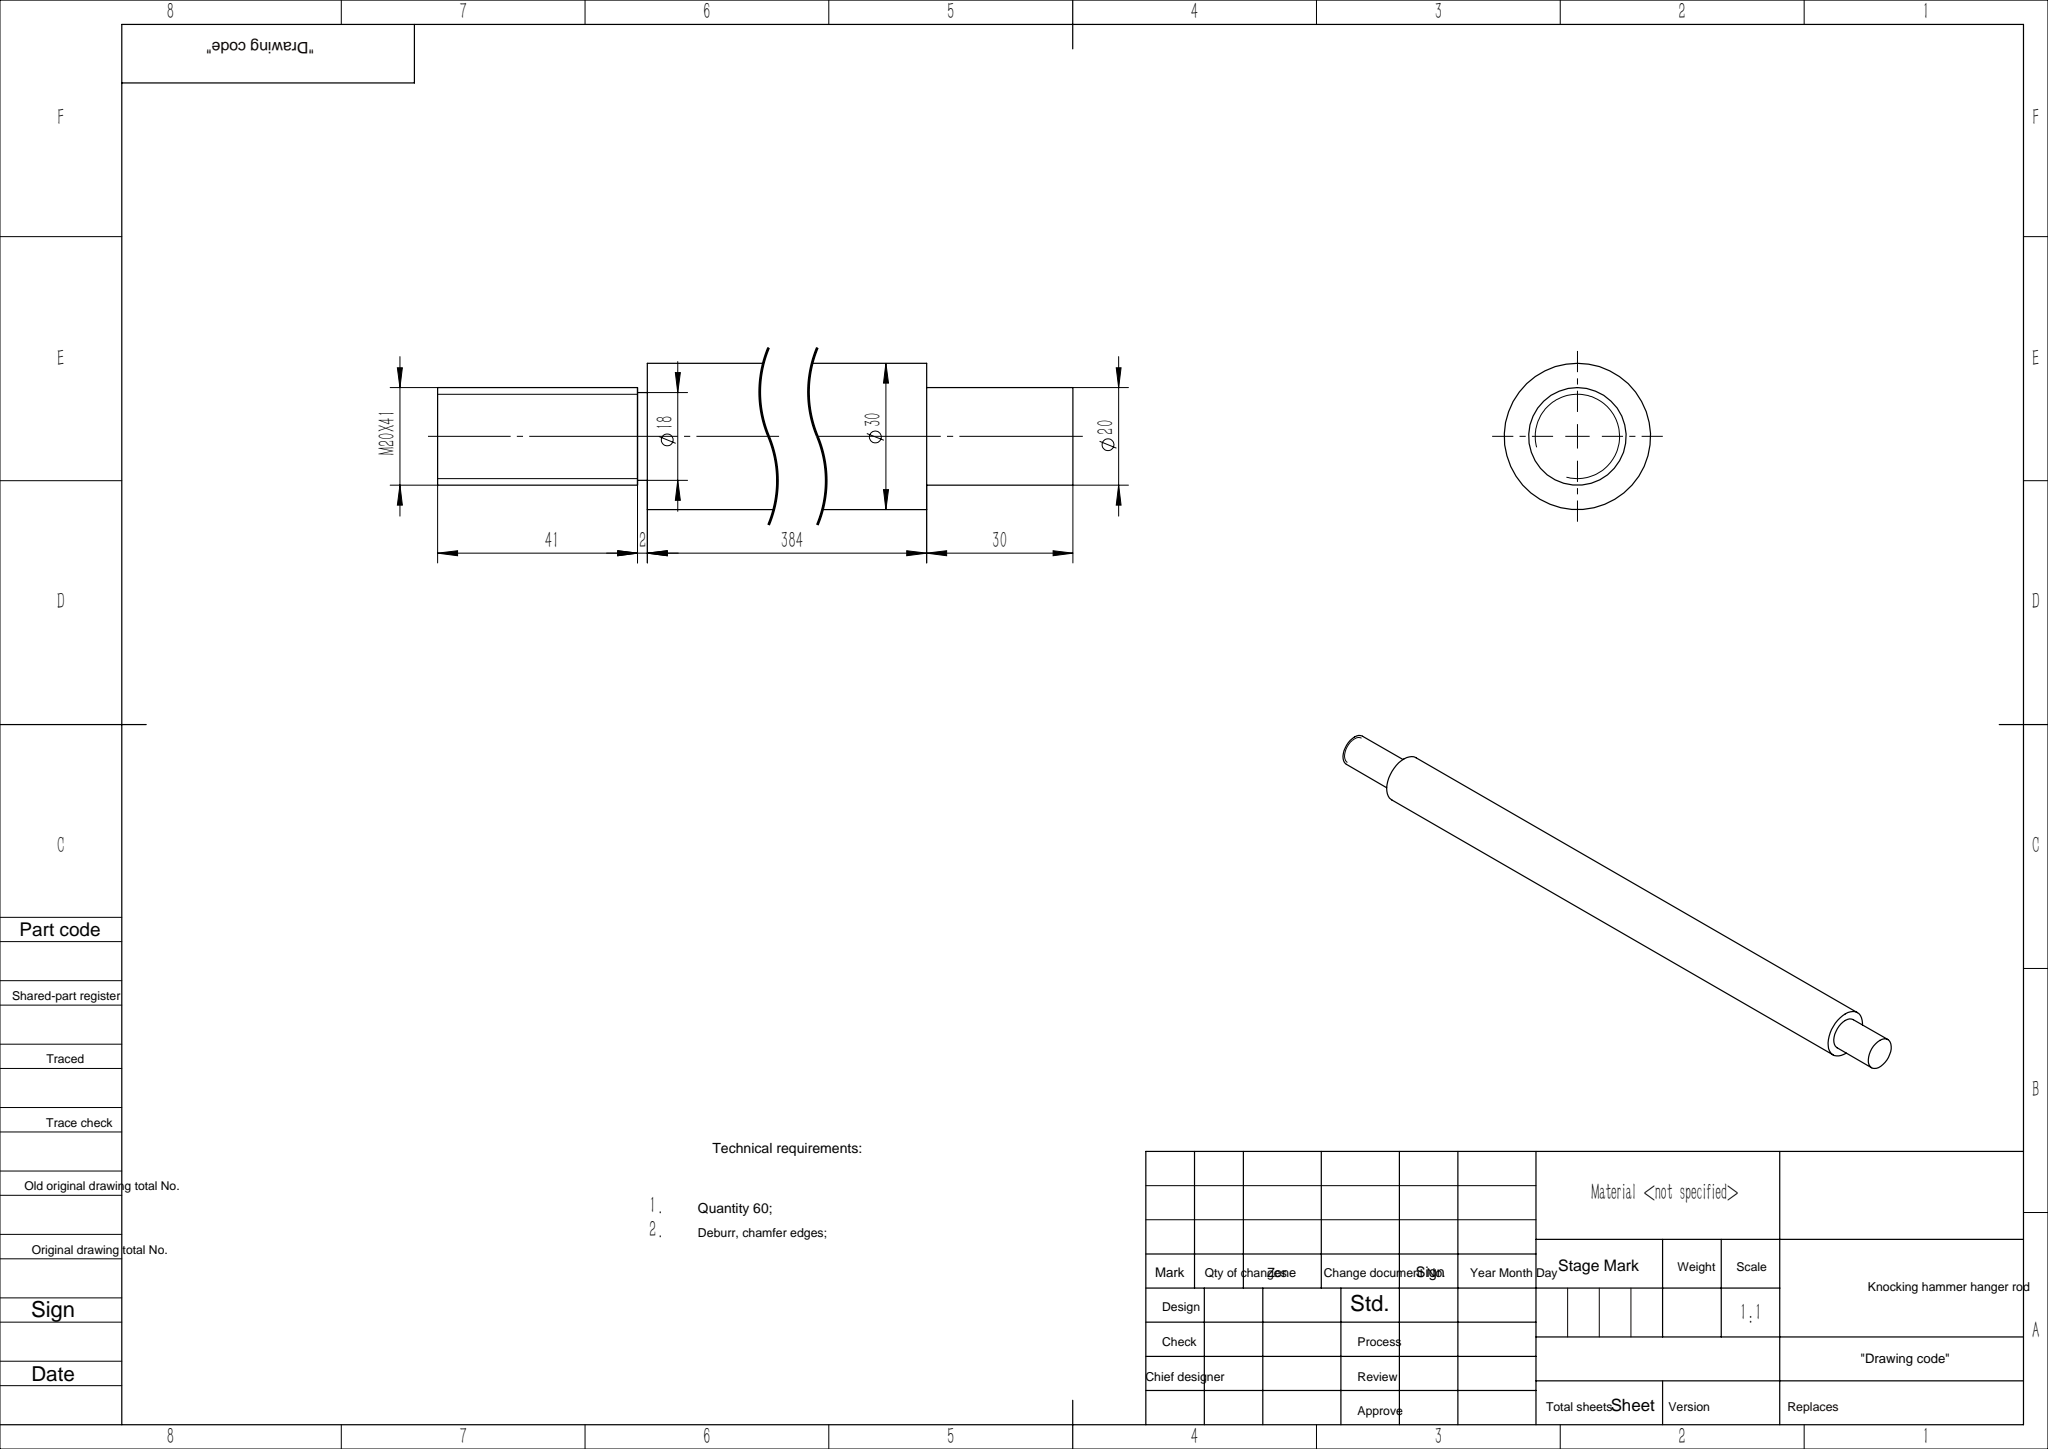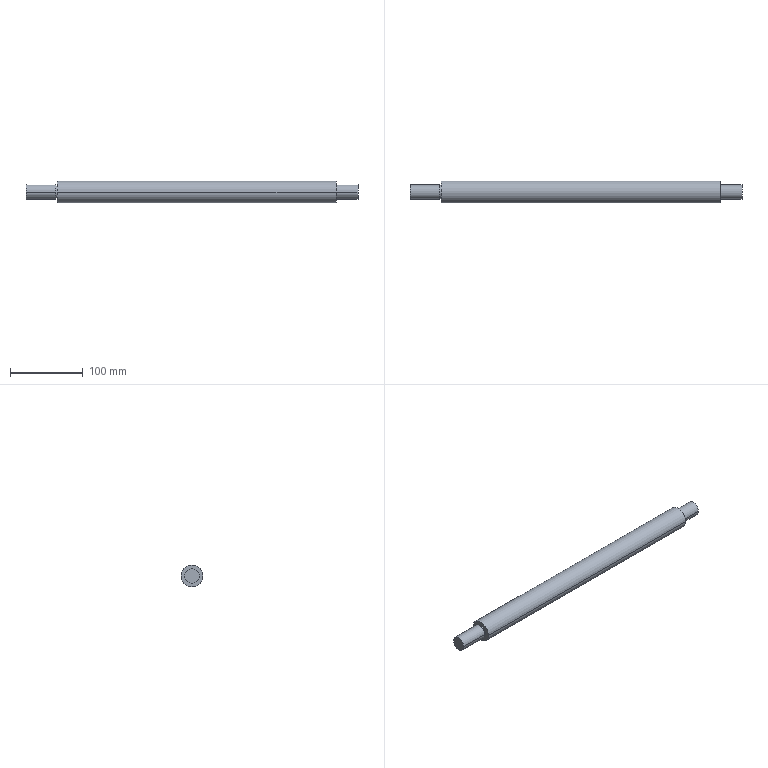Part | SolidWorks | features ICE 1, Revolution 1 | 1 solid | 13 faces | box 457 x 30 x 30 mm | volume 294248 mm3 | cylinder 8 | plane 5 | commonest cylinder face diameters 20 x4 18 x2 30 x2
STEP:
#1=CARTESIAN_POINT('',(0.,10.,0.));
#2=VERTEX_POINT('',#1);
#3=CARTESIAN_POINT('',(0.,-10.,0.));
#4=VERTEX_POINT('',#3);
#5=CARTESIAN_POINT('',(0.,0.,0.));
#6=DIRECTION('',(1.,0.,0.));
#7=DIRECTION('',(0.,1.,0.));
#8=AXIS2_PLACEMENT_3D('',#5,#6,#7);
#9=CIRCLE('',#8,10.);
#10=EDGE_CURVE('',#2,#4,#9,.T.);
#11=ORIENTED_EDGE('',*,*,#10,.T.);
#12=CARTESIAN_POINT('',(41.,-10.,0.));
#13=VERTEX_POINT('',#12);
#14=CARTESIAN_POINT('',(457.,-10.,0.));
#15=DIRECTION('',(1.,0.,0.));
#16=VECTOR('',#15,1000.);
#17=LINE('',#14,#16);
#18=EDGE_CURVE('',#4,#13,#17,.T.);
#19=ORIENTED_EDGE('',*,*,#18,.T.);
#20=CARTESIAN_POINT('',(41.,10.,0.));
#21=VERTEX_POINT('',#20);
#22=CARTESIAN_POINT('',(41.,0.,0.));
#23=DIRECTION('',(-1.,0.,0.));
#24=DIRECTION('',(0.,-1.,0.));
#25=AXIS2_PLACEMENT_3D('',#22,#23,#24);
#26=CIRCLE('',#25,10.);
#27=EDGE_CURVE('',#13,#21,#26,.T.);
#28=ORIENTED_EDGE('',*,*,#27,.T.);
#29=CARTESIAN_POINT('',(457.,10.,0.));
#30=DIRECTION('',(1.,0.,0.));
#31=VECTOR('',#30,1000.);
#32=LINE('',#29,#31);
#33=EDGE_CURVE('',#2,#21,#32,.T.);
#34=ORIENTED_EDGE('',*,*,#33,.F.);
#35=EDGE_LOOP('',(#11,#19,#28,#34));
#36=FACE_OUTER_BOUND('',#35,.T.);
#37=CARTESIAN_POINT('',(457.,0.,0.));
#38=DIRECTION('',(1.,0.,0.));
#39=DIRECTION('',(0.,1.,0.));
#40=AXIS2_PLACEMENT_3D('',#37,#38,#39);
#41=CYLINDRICAL_SURFACE('',#40,10.);
#42=ADVANCED_FACE('',(#36),#41,.T.);
#43=CARTESIAN_POINT('',(41.,-9.,0.));
#44=VERTEX_POINT('',#43);
#45=CARTESIAN_POINT('',(41.,9.,0.));
#46=VERTEX_POINT('',#45);
#47=CARTESIAN_POINT('',(41.,0.,0.));
#48=DIRECTION('',(-1.,0.,0.));
#49=DIRECTION('',(0.,-1.,0.));
#50=AXIS2_PLACEMENT_3D('',#47,#48,#49);
#51=CIRCLE('',#50,9.);
#52=EDGE_CURVE('',#44,#46,#51,.T.);
#53=ORIENTED_EDGE('',*,*,#52,.F.);
#54=CARTESIAN_POINT('',(43.,-9.,0.));
#55=VERTEX_POINT('',#54);
#56=CARTESIAN_POINT('',(41.,-9.,0.));
#57=DIRECTION('',(1.,0.,0.));
#58=VECTOR('',#57,1000.);
#59=LINE('',#56,#58);
#60=EDGE_CURVE('',#44,#55,#59,.T.);
#61=ORIENTED_EDGE('',*,*,#60,.T.);
#62=CARTESIAN_POINT('',(43.,9.,0.));
#63=VERTEX_POINT('',#62);
#64=CARTESIAN_POINT('',(43.,0.,0.));
#65=DIRECTION('',(-1.,0.,0.));
#66=DIRECTION('',(0.,-1.,0.));
#67=AXIS2_PLACEMENT_3D('',#64,#65,#66);
#68=CIRCLE('',#67,9.);
#69=EDGE_CURVE('',#55,#63,#68,.T.);
#70=ORIENTED_EDGE('',*,*,#69,.T.);
#71=CARTESIAN_POINT('',(41.,9.,0.));
#72=DIRECTION('',(1.,0.,0.));
#73=VECTOR('',#72,1000.);
#74=LINE('',#71,#73);
#75=EDGE_CURVE('',#46,#63,#74,.T.);
#76=ORIENTED_EDGE('',*,*,#75,.F.);
#77=EDGE_LOOP('',(#53,#61,#70,#76));
#78=FACE_OUTER_BOUND('',#77,.T.);
#79=CARTESIAN_POINT('',(41.,0.,0.));
#80=DIRECTION('',(1.,0.,0.));
#81=DIRECTION('',(0.,1.,0.));
#82=AXIS2_PLACEMENT_3D('',#79,#80,#81);
#83=CYLINDRICAL_SURFACE('',#82,9.);
#84=ADVANCED_FACE('',(#78),#83,.T.);
#85=CARTESIAN_POINT('',(427.,10.,0.));
#86=VERTEX_POINT('',#85);
#87=CARTESIAN_POINT('',(427.,-10.,0.));
#88=VERTEX_POINT('',#87);
#89=CARTESIAN_POINT('',(427.,0.,0.));
#90=DIRECTION('',(1.,0.,0.));
#91=DIRECTION('',(0.,1.,0.));
#92=AXIS2_PLACEMENT_3D('',#89,#90,#91);
#93=CIRCLE('',#92,10.);
#94=EDGE_CURVE('',#86,#88,#93,.T.);
#95=ORIENTED_EDGE('',*,*,#94,.T.);
#96=CARTESIAN_POINT('',(457.,-10.,0.));
#97=VERTEX_POINT('',#96);
#98=CARTESIAN_POINT('',(457.,-10.,0.));
#99=DIRECTION('',(1.,0.,0.));
#100=VECTOR('',#99,1000.);
#101=LINE('',#98,#100);
#102=EDGE_CURVE('',#88,#97,#101,.T.);
#103=ORIENTED_EDGE('',*,*,#102,.T.);
#104=CARTESIAN_POINT('',(457.,10.,0.));
#105=VERTEX_POINT('',#104);
#106=CARTESIAN_POINT('',(457.,0.,0.));
#107=DIRECTION('',(1.,0.,0.));
#108=DIRECTION('',(0.,1.,0.));
#109=AXIS2_PLACEMENT_3D('',#106,#107,#108);
#110=CIRCLE('',#109,10.);
#111=EDGE_CURVE('',#105,#97,#110,.T.);
#112=ORIENTED_EDGE('',*,*,#111,.F.);
#113=CARTESIAN_POINT('',(457.,10.,0.));
#114=DIRECTION('',(1.,0.,0.));
#115=VECTOR('',#114,1000.);
#116=LINE('',#113,#115);
#117=EDGE_CURVE('',#86,#105,#116,.T.);
#118=ORIENTED_EDGE('',*,*,#117,.F.);
#119=EDGE_LOOP('',(#95,#103,#112,#118));
#120=FACE_OUTER_BOUND('',#119,.T.);
#121=CARTESIAN_POINT('',(457.,0.,0.));
#122=DIRECTION('',(1.,0.,0.));
#123=DIRECTION('',(0.,1.,0.));
#124=AXIS2_PLACEMENT_3D('',#121,#122,#123);
#125=CYLINDRICAL_SURFACE('',#124,10.);
#126=ADVANCED_FACE('',(#120),#125,.T.);
#127=CARTESIAN_POINT('',(43.,15.,0.));
#128=VERTEX_POINT('',#127);
#129=CARTESIAN_POINT('',(43.,-15.,0.));
#130=VERTEX_POINT('',#129);
#131=CARTESIAN_POINT('',(43.,0.,0.));
#132=DIRECTION('',(1.,0.,0.));
#133=DIRECTION('',(0.,1.,0.));
#134=AXIS2_PLACEMENT_3D('',#131,#132,#133);
#135=CIRCLE('',#134,15.);
#136=EDGE_CURVE('',#128,#130,#135,.T.);
#137=ORIENTED_EDGE('',*,*,#136,.T.);
#138=CARTESIAN_POINT('',(427.,-15.,0.));
#139=VERTEX_POINT('',#138);
#140=CARTESIAN_POINT('',(457.,-15.,0.));
#141=DIRECTION('',(1.,0.,0.));
#142=VECTOR('',#141,1000.);
#143=LINE('',#140,#142);
#144=EDGE_CURVE('',#130,#139,#143,.T.);
#145=ORIENTED_EDGE('',*,*,#144,.T.);
#146=CARTESIAN_POINT('',(427.,15.,0.));
#147=VERTEX_POINT('',#146);
#148=CARTESIAN_POINT('',(427.,0.,0.));
#149=DIRECTION('',(1.,0.,0.));
#150=DIRECTION('',(0.,1.,0.));
#151=AXIS2_PLACEMENT_3D('',#148,#149,#150);
#152=CIRCLE('',#151,15.);
#153=EDGE_CURVE('',#147,#139,#152,.T.);
#154=ORIENTED_EDGE('',*,*,#153,.F.);
#155=CARTESIAN_POINT('',(457.,15.,0.));
#156=DIRECTION('',(1.,0.,0.));
#157=VECTOR('',#156,1000.);
#158=LINE('',#155,#157);
#159=EDGE_CURVE('',#128,#147,#158,.T.);
#160=ORIENTED_EDGE('',*,*,#159,.F.);
#161=EDGE_LOOP('',(#137,#145,#154,#160));
#162=FACE_OUTER_BOUND('',#161,.T.);
#163=CARTESIAN_POINT('',(457.,0.,0.));
#164=DIRECTION('',(1.,0.,0.));
#165=DIRECTION('',(0.,1.,0.));
#166=AXIS2_PLACEMENT_3D('',#163,#164,#165);
#167=CYLINDRICAL_SURFACE('',#166,15.);
#168=ADVANCED_FACE('',(#162),#167,.T.);
#169=ORIENTED_EDGE('',*,*,#136,.F.);
#170=CARTESIAN_POINT('',(43.,0.,0.));
#171=DIRECTION('',(1.,0.,0.));
#172=DIRECTION('',(0.,1.,0.));
#173=AXIS2_PLACEMENT_3D('',#170,#171,#172);
#174=CIRCLE('',#173,15.);
#175=EDGE_CURVE('',#130,#128,#174,.T.);
#176=ORIENTED_EDGE('',*,*,#175,.F.);
#177=EDGE_LOOP('',(#169,#176));
#178=FACE_OUTER_BOUND('',#177,.T.);
#179=CARTESIAN_POINT('',(43.,0.,0.));
#180=DIRECTION('',(-1.,0.,0.));
#181=DIRECTION('',(0.,-1.,0.));
#182=AXIS2_PLACEMENT_3D('',#179,#180,#181);
#183=CIRCLE('',#182,9.);
#184=EDGE_CURVE('',#63,#55,#183,.T.);
#185=ORIENTED_EDGE('',*,*,#184,.F.);
#186=ORIENTED_EDGE('',*,*,#69,.F.);
#187=EDGE_LOOP('',(#185,#186));
#188=FACE_BOUND('',#187,.T.);
#189=CARTESIAN_POINT('',(43.,10.,0.));
#190=DIRECTION('',(-1.,0.,0.));
#191=DIRECTION('',(0.,-1.,0.));
#192=AXIS2_PLACEMENT_3D('',#189,#190,#191);
#193=PLANE('',#192);
#194=ADVANCED_FACE('',(#178,#188),#193,.T.);
#195=ORIENTED_EDGE('',*,*,#144,.F.);
#196=ORIENTED_EDGE('',*,*,#175,.T.);
#197=ORIENTED_EDGE('',*,*,#159,.T.);
#198=CARTESIAN_POINT('',(427.,0.,0.));
#199=DIRECTION('',(1.,0.,0.));
#200=DIRECTION('',(0.,1.,0.));
#201=AXIS2_PLACEMENT_3D('',#198,#199,#200);
#202=CIRCLE('',#201,15.);
#203=EDGE_CURVE('',#139,#147,#202,.T.);
#204=ORIENTED_EDGE('',*,*,#203,.F.);
#205=EDGE_LOOP('',(#195,#196,#197,#204));
#206=FACE_OUTER_BOUND('',#205,.T.);
#207=CARTESIAN_POINT('',(457.,0.,0.));
#208=DIRECTION('',(1.,0.,0.));
#209=DIRECTION('',(0.,1.,0.));
#210=AXIS2_PLACEMENT_3D('',#207,#208,#209);
#211=CYLINDRICAL_SURFACE('',#210,15.);
#212=ADVANCED_FACE('',(#206),#211,.T.);
#213=ORIENTED_EDGE('',*,*,#153,.T.);
#214=ORIENTED_EDGE('',*,*,#203,.T.);
#215=EDGE_LOOP('',(#213,#214));
#216=FACE_OUTER_BOUND('',#215,.T.);
#217=ORIENTED_EDGE('',*,*,#94,.F.);
#218=CARTESIAN_POINT('',(427.,0.,0.));
#219=DIRECTION('',(1.,0.,0.));
#220=DIRECTION('',(0.,1.,0.));
#221=AXIS2_PLACEMENT_3D('',#218,#219,#220);
#222=CIRCLE('',#221,10.);
#223=EDGE_CURVE('',#88,#86,#222,.T.);
#224=ORIENTED_EDGE('',*,*,#223,.F.);
#225=EDGE_LOOP('',(#217,#224));
#226=FACE_BOUND('',#225,.T.);
#227=CARTESIAN_POINT('',(427.,15.,0.));
#228=DIRECTION('',(1.,0.,0.));
#229=DIRECTION('',(0.,1.,0.));
#230=AXIS2_PLACEMENT_3D('',#227,#228,#229);
#231=PLANE('',#230);
#232=ADVANCED_FACE('',(#216,#226),#231,.T.);
#233=ORIENTED_EDGE('',*,*,#102,.F.);
#234=ORIENTED_EDGE('',*,*,#223,.T.);
#235=ORIENTED_EDGE('',*,*,#117,.T.);
#236=CARTESIAN_POINT('',(457.,0.,0.));
#237=DIRECTION('',(1.,0.,0.));
#238=DIRECTION('',(0.,1.,0.));
#239=AXIS2_PLACEMENT_3D('',#236,#237,#238);
#240=CIRCLE('',#239,10.);
#241=EDGE_CURVE('',#97,#105,#240,.T.);
#242=ORIENTED_EDGE('',*,*,#241,.F.);
#243=EDGE_LOOP('',(#233,#234,#235,#242));
#244=FACE_OUTER_BOUND('',#243,.T.);
#245=CARTESIAN_POINT('',(457.,0.,0.));
#246=DIRECTION('',(1.,0.,0.));
#247=DIRECTION('',(0.,1.,0.));
#248=AXIS2_PLACEMENT_3D('',#245,#246,#247);
#249=CYLINDRICAL_SURFACE('',#248,10.);
#250=ADVANCED_FACE('',(#244),#249,.T.);
#251=ORIENTED_EDGE('',*,*,#111,.T.);
#252=ORIENTED_EDGE('',*,*,#241,.T.);
#253=EDGE_LOOP('',(#251,#252));
#254=FACE_OUTER_BOUND('',#253,.T.);
#255=CARTESIAN_POINT('',(457.,10.,0.));
#256=DIRECTION('',(1.,0.,0.));
#257=DIRECTION('',(0.,1.,0.));
#258=AXIS2_PLACEMENT_3D('',#255,#256,#257);
#259=PLANE('',#258);
#260=ADVANCED_FACE('',(#254),#259,.T.);
#261=CARTESIAN_POINT('',(41.,0.,0.));
#262=DIRECTION('',(-1.,0.,0.));
#263=DIRECTION('',(0.,-1.,0.));
#264=AXIS2_PLACEMENT_3D('',#261,#262,#263);
#265=CIRCLE('',#264,10.);
#266=EDGE_CURVE('',#21,#13,#265,.T.);
#267=ORIENTED_EDGE('',*,*,#266,.F.);
#268=ORIENTED_EDGE('',*,*,#27,.F.);
#269=EDGE_LOOP('',(#267,#268));
#270=FACE_OUTER_BOUND('',#269,.T.);
#271=CARTESIAN_POINT('',(41.,0.,0.));
#272=DIRECTION('',(-1.,0.,0.));
#273=DIRECTION('',(0.,-1.,0.));
#274=AXIS2_PLACEMENT_3D('',#271,#272,#273);
#275=CIRCLE('',#274,9.);
#276=EDGE_CURVE('',#46,#44,#275,.T.);
#277=ORIENTED_EDGE('',*,*,#276,.T.);
#278=ORIENTED_EDGE('',*,*,#52,.T.);
#279=EDGE_LOOP('',(#277,#278));
#280=FACE_BOUND('',#279,.T.);
#281=CARTESIAN_POINT('',(41.,0.,0.));
#282=DIRECTION('',(-1.,0.,0.));
#283=DIRECTION('',(0.,-1.,0.));
#284=AXIS2_PLACEMENT_3D('',#281,#282,#283);
#285=PLANE('',#284);
#286=ADVANCED_FACE('',(#270,#280),#285,.F.);
#287=ORIENTED_EDGE('',*,*,#60,.F.);
#288=ORIENTED_EDGE('',*,*,#276,.F.);
#289=ORIENTED_EDGE('',*,*,#75,.T.);
#290=ORIENTED_EDGE('',*,*,#184,.T.);
#291=EDGE_LOOP('',(#287,#288,#289,#290));
#292=FACE_OUTER_BOUND('',#291,.T.);
#293=CARTESIAN_POINT('',(41.,0.,0.));
#294=DIRECTION('',(1.,0.,0.));
#295=DIRECTION('',(0.,1.,0.));
#296=AXIS2_PLACEMENT_3D('',#293,#294,#295);
#297=CYLINDRICAL_SURFACE('',#296,9.);
#298=ADVANCED_FACE('',(#292),#297,.T.);
#299=ORIENTED_EDGE('',*,*,#10,.F.);
#300=CARTESIAN_POINT('',(0.,0.,0.));
#301=DIRECTION('',(1.,0.,0.));
#302=DIRECTION('',(0.,1.,0.));
#303=AXIS2_PLACEMENT_3D('',#300,#301,#302);
#304=CIRCLE('',#303,10.);
#305=EDGE_CURVE('',#4,#2,#304,.T.);
#306=ORIENTED_EDGE('',*,*,#305,.F.);
#307=EDGE_LOOP('',(#299,#306));
#308=FACE_OUTER_BOUND('',#307,.T.);
#309=CARTESIAN_POINT('',(0.,0.,0.));
#310=DIRECTION('',(-1.,0.,0.));
#311=DIRECTION('',(0.,-1.,0.));
#312=AXIS2_PLACEMENT_3D('',#309,#310,#311);
#313=PLANE('',#312);
#314=ADVANCED_FACE('',(#308),#313,.T.);
#315=ORIENTED_EDGE('',*,*,#18,.F.);
#316=ORIENTED_EDGE('',*,*,#305,.T.);
#317=ORIENTED_EDGE('',*,*,#33,.T.);
#318=ORIENTED_EDGE('',*,*,#266,.T.);
#319=EDGE_LOOP('',(#315,#316,#317,#318));
#320=FACE_OUTER_BOUND('',#319,.T.);
#321=CARTESIAN_POINT('',(457.,0.,0.));
#322=DIRECTION('',(1.,0.,0.));
#323=DIRECTION('',(0.,1.,0.));
#324=AXIS2_PLACEMENT_3D('',#321,#322,#323);
#325=CYLINDRICAL_SURFACE('',#324,10.);
#326=ADVANCED_FACE('',(#320),#325,.T.);
#327=CLOSED_SHELL('',(#42,#84,#126,#168,#194,#212,#232,#250,#260,#286,#298,#314,#326));
#328=MANIFOLD_SOLID_BREP('',#327);
#329=CARTESIAN_POINT('',(0.,0.,0.));
#330=DIRECTION('',(0.,0.,1.));
#331=DIRECTION('',(1.,0.,0.));
#332=AXIS2_PLACEMENT_3D('',#329,#330,#331);
#333=(LENGTH_UNIT()NAMED_UNIT(*)SI_UNIT(.MILLI.,.METRE.));
#334=UNCERTAINTY_MEASURE_WITH_UNIT(LENGTH_MEASURE(0.00001),#333,'','');
#335=(NAMED_UNIT(*)PLANE_ANGLE_UNIT()SI_UNIT($,.RADIAN.));
#336=(NAMED_UNIT(*)SI_UNIT($,.STERADIAN.)SOLID_ANGLE_UNIT());
#337=(GEOMETRIC_REPRESENTATION_CONTEXT(3)GLOBAL_UNCERTAINTY_ASSIGNED_CONTEXT((#334))GLOBAL_UNIT_ASSIGNED_CONTEXT((#333,#335,#336))REPRESENTATION_CONTEXT('',''));
#338=ADVANCED_BREP_SHAPE_REPRESENTATION('',(#328,#332),#337);